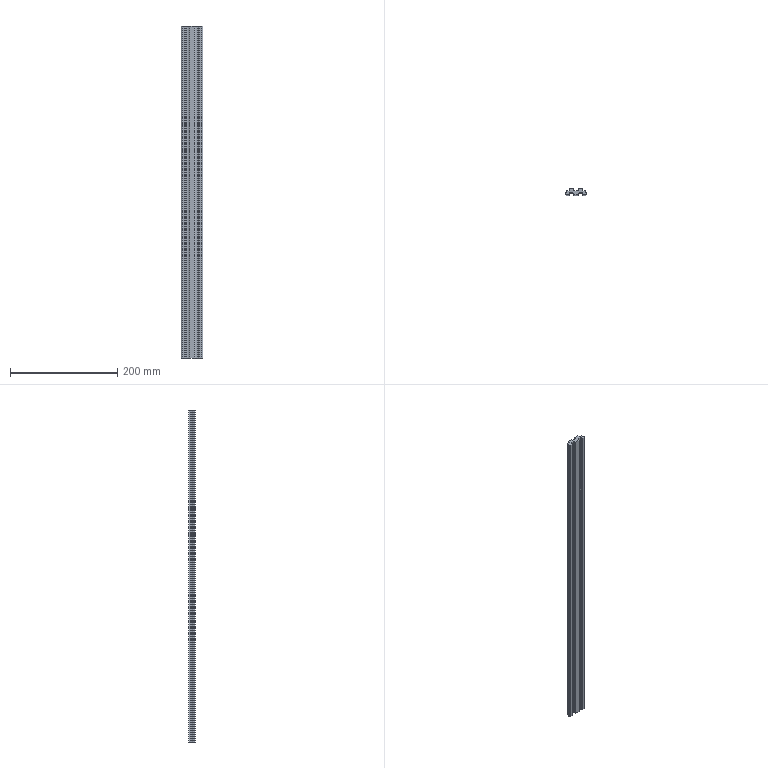Part | STEP file | 1 solid | 46 faces | box 41 x 12 x 620 mm | volume 198150 mm3 | plane 28 | cylinder 18 | commonest cylinder face diameters 1 x12 4 x4 2 x2